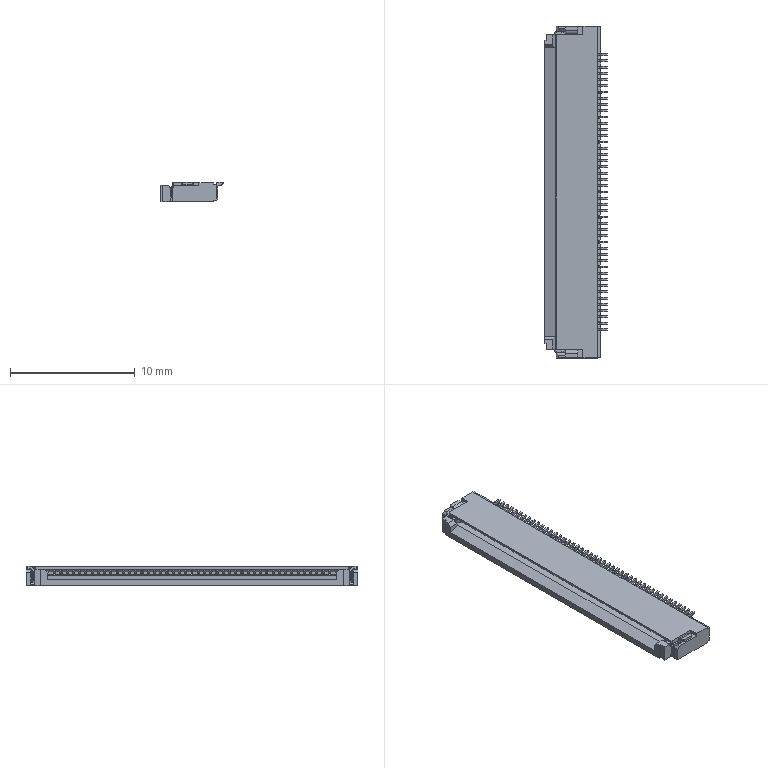Part | Creo | 1 solid | 3585 faces | volume 114.548 mm3 | plane 2387 | cylinder 1198 | commonest cylinder face diameters 0.2 x415 0.1 x142 0.6 x137 0.3 x135 0.15 x90 0.241 x90